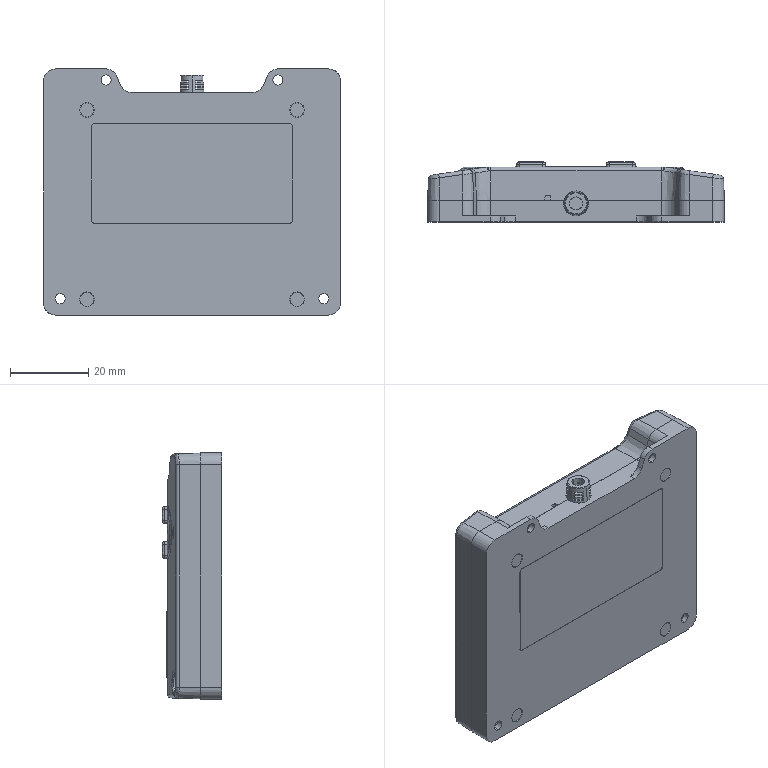Part | SolidWorks | features BaseBody 13, DeleteBody 1, Revolution 1 | 10 solids | 2017 faces | box 76 x 15.355 x 63 mm | volume 45153 mm3 | plane 1090 | cylinder 512 | spline 214 | cone 201 | commonest cylinder face diameters 2 x113 1.8 x56 1 x40 6 x36 0.4 x21 4 x19